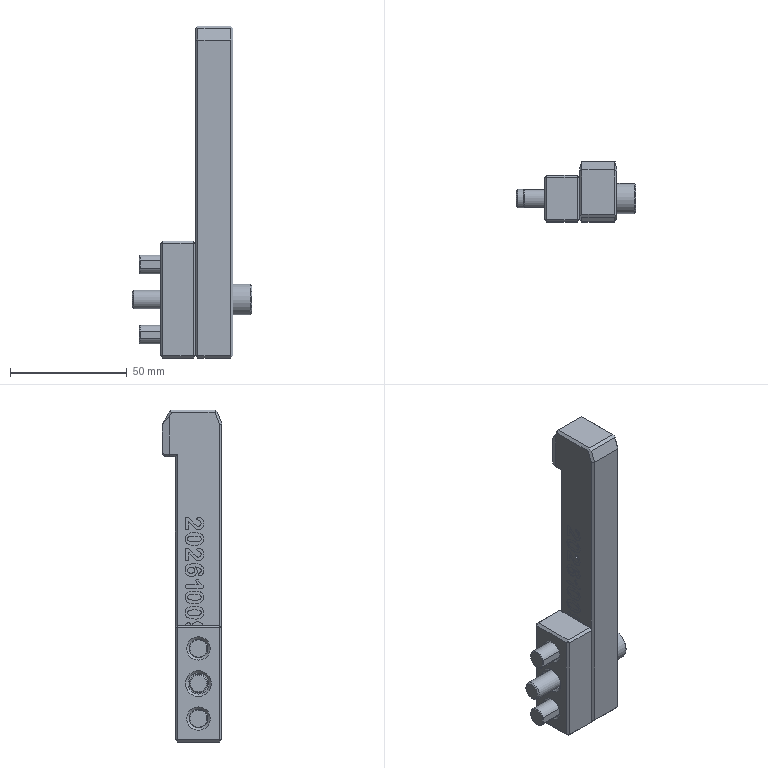Part | NX | features BREP 22, solid 10, CHAMFER 9, SUBTRACT 5 | 5 solids | 288 faces | box 51 x 25.5 x 142 mm | volume 62882 mm3 | plane 137 | spline 115 | cone 22 | cylinder 14 | commonest cylinder face diameters 8 x7 3.2 x2 4 x2 9 x2 13 x1